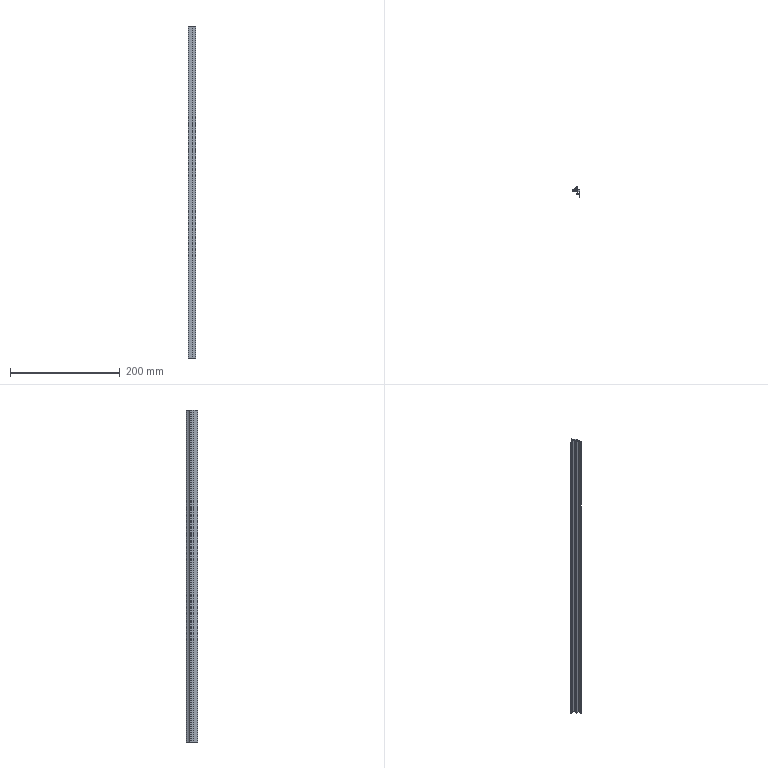Part | SolidWorks | features BaseBody 1, ICE 1, MoveFace 1 | 1 solid | 27 faces | box 14 x 20.3 x 606 mm | volume 30855 mm3 | plane 20 | cylinder 7 | commonest cylinder face diameters 0.387 x2 0.8 x2 0.4 x1 20 x1 22 x1
STEP:
#1=CARTESIAN_POINT('',(-5.304,-0.625,200.));
#2=VERTEX_POINT('',#1);
#3=CARTESIAN_POINT('',(-5.449,-0.8125,200.));
#4=VERTEX_POINT('',#3);
#5=CARTESIAN_POINT('',(-5.255,-0.8125,200.));
#6=DIRECTION('',(0.,0.,1.));
#7=DIRECTION('',(-1.,0.,0.));
#8=AXIS2_PLACEMENT_3D('',#5,#6,#7);
#9=CIRCLE('',#8,0.1937);
#10=EDGE_CURVE('',#2,#4,#9,.T.);
#11=ORIENTED_EDGE('',*,*,#10,.T.);
#12=CARTESIAN_POINT('',(-5.449,-0.8125,-406.));
#13=VERTEX_POINT('',#12);
#14=CARTESIAN_POINT('',(-5.449,-0.8125,230.));
#15=DIRECTION('',(0.,0.,-1.));
#16=VECTOR('',#15,1000.);
#17=LINE('',#14,#16);
#18=EDGE_CURVE('',#4,#13,#17,.T.);
#19=ORIENTED_EDGE('',*,*,#18,.T.);
#20=CARTESIAN_POINT('',(-5.304,-0.625,-406.));
#21=VERTEX_POINT('',#20);
#22=CARTESIAN_POINT('',(-5.255,-0.8125,-406.));
#23=DIRECTION('',(0.,0.,-1.));
#24=DIRECTION('',(1.,0.,0.));
#25=AXIS2_PLACEMENT_3D('',#22,#23,#24);
#26=CIRCLE('',#25,0.1937);
#27=EDGE_CURVE('',#13,#21,#26,.T.);
#28=ORIENTED_EDGE('',*,*,#27,.T.);
#29=CARTESIAN_POINT('',(-5.304,-0.625,230.));
#30=DIRECTION('',(0.,0.,-1.));
#31=VECTOR('',#30,1000.);
#32=LINE('',#29,#31);
#33=EDGE_CURVE('',#2,#21,#32,.T.);
#34=ORIENTED_EDGE('',*,*,#33,.F.);
#35=EDGE_LOOP('',(#11,#19,#28,#34));
#36=FACE_OUTER_BOUND('',#35,.T.);
#37=CARTESIAN_POINT('',(-5.255,-0.8125,230.));
#38=DIRECTION('',(0.,0.,-1.));
#39=DIRECTION('',(-1.,0.,0.));
#40=AXIS2_PLACEMENT_3D('',#37,#38,#39);
#41=CYLINDRICAL_SURFACE('',#40,0.1937);
#42=ADVANCED_FACE('',(#36),#41,.F.);
#43=CARTESIAN_POINT('',(5.,-1.,-406.));
#44=VERTEX_POINT('',#43);
#45=CARTESIAN_POINT('',(5.,-14.3,-406.));
#46=VERTEX_POINT('',#45);
#47=CARTESIAN_POINT('',(5.,29.623,-406.));
#48=DIRECTION('',(0.,-1.,0.));
#49=VECTOR('',#48,1000.);
#50=LINE('',#47,#49);
#51=EDGE_CURVE('',#44,#46,#50,.T.);
#52=ORIENTED_EDGE('',*,*,#51,.F.);
#53=CARTESIAN_POINT('',(5.,-1.,200.));
#54=VERTEX_POINT('',#53);
#55=CARTESIAN_POINT('',(5.,-1.,230.));
#56=DIRECTION('',(0.,0.,-1.));
#57=VECTOR('',#56,1000.);
#58=LINE('',#55,#57);
#59=EDGE_CURVE('',#54,#44,#58,.T.);
#60=ORIENTED_EDGE('',*,*,#59,.F.);
#61=CARTESIAN_POINT('',(5.,-14.3,200.));
#62=VERTEX_POINT('',#61);
#63=CARTESIAN_POINT('',(5.,-14.3,200.));
#64=DIRECTION('',(0.,1.,0.));
#65=VECTOR('',#64,1000.);
#66=LINE('',#63,#65);
#67=EDGE_CURVE('',#62,#54,#66,.T.);
#68=ORIENTED_EDGE('',*,*,#67,.F.);
#69=CARTESIAN_POINT('',(5.,-14.3,230.));
#70=DIRECTION('',(0.,0.,1.));
#71=VECTOR('',#70,1000.);
#72=LINE('',#69,#71);
#73=EDGE_CURVE('',#46,#62,#72,.T.);
#74=ORIENTED_EDGE('',*,*,#73,.F.);
#75=EDGE_LOOP('',(#52,#60,#68,#74));
#76=FACE_OUTER_BOUND('',#75,.T.);
#77=CARTESIAN_POINT('',(5.,-14.3,230.));
#78=DIRECTION('',(-1.,0.,0.));
#79=DIRECTION('',(0.,0.,1.));
#80=AXIS2_PLACEMENT_3D('',#77,#78,#79);
#81=PLANE('',#80);
#82=ADVANCED_FACE('',(#76),#81,.F.);
#83=CARTESIAN_POINT('',(-9.,-2.,-406.));
#84=VERTEX_POINT('',#83);
#85=CARTESIAN_POINT('',(-9.,-2.,200.));
#86=VERTEX_POINT('',#85);
#87=CARTESIAN_POINT('',(-9.,-2.,230.));
#88=DIRECTION('',(0.,0.,1.));
#89=VECTOR('',#88,1000.);
#90=LINE('',#87,#89);
#91=EDGE_CURVE('',#84,#86,#90,.T.);
#92=ORIENTED_EDGE('',*,*,#91,.F.);
#93=CARTESIAN_POINT('',(0.9,-2.,-406.));
#94=VERTEX_POINT('',#93);
#95=CARTESIAN_POINT('',(5.,-2.,-406.));
#96=DIRECTION('',(-1.,0.,0.));
#97=VECTOR('',#96,1000.);
#98=LINE('',#95,#97);
#99=EDGE_CURVE('',#94,#84,#98,.T.);
#100=ORIENTED_EDGE('',*,*,#99,.F.);
#101=CARTESIAN_POINT('',(0.9,-2.,200.));
#102=VERTEX_POINT('',#101);
#103=CARTESIAN_POINT('',(0.9,-2.,230.));
#104=DIRECTION('',(0.,0.,-1.));
#105=VECTOR('',#104,1000.);
#106=LINE('',#103,#105);
#107=EDGE_CURVE('',#102,#94,#106,.T.);
#108=ORIENTED_EDGE('',*,*,#107,.F.);
#109=CARTESIAN_POINT('',(5.,-2.,200.));
#110=DIRECTION('',(1.,0.,0.));
#111=VECTOR('',#110,1000.);
#112=LINE('',#109,#111);
#113=EDGE_CURVE('',#86,#102,#112,.T.);
#114=ORIENTED_EDGE('',*,*,#113,.F.);
#115=EDGE_LOOP('',(#92,#100,#108,#114));
#116=FACE_OUTER_BOUND('',#115,.T.);
#117=CARTESIAN_POINT('',(-9.,-2.,230.));
#118=DIRECTION('',(0.,1.,0.));
#119=DIRECTION('',(0.,0.,1.));
#120=AXIS2_PLACEMENT_3D('',#117,#118,#119);
#121=PLANE('',#120);
#122=ADVANCED_FACE('',(#116),#121,.F.);
#123=CARTESIAN_POINT('',(4.,-6.,200.));
#124=VERTEX_POINT('',#123);
#125=CARTESIAN_POINT('',(4.,-3.,200.));
#126=VERTEX_POINT('',#125);
#127=CARTESIAN_POINT('',(4.,29.623,200.));
#128=DIRECTION('',(0.,1.,0.));
#129=VECTOR('',#128,1000.);
#130=LINE('',#127,#129);
#131=EDGE_CURVE('',#124,#126,#130,.T.);
#132=ORIENTED_EDGE('',*,*,#131,.F.);
#133=CARTESIAN_POINT('',(1.,-6.,200.));
#134=VERTEX_POINT('',#133);
#135=CARTESIAN_POINT('',(5.,-6.,200.));
#136=DIRECTION('',(1.,0.,0.));
#137=VECTOR('',#136,1000.);
#138=LINE('',#135,#137);
#139=EDGE_CURVE('',#134,#124,#138,.T.);
#140=ORIENTED_EDGE('',*,*,#139,.F.);
#141=CARTESIAN_POINT('',(1.,-6.7,200.));
#142=VERTEX_POINT('',#141);
#143=CARTESIAN_POINT('',(1.,-6.,200.));
#144=DIRECTION('',(0.,-1.,0.));
#145=VECTOR('',#144,1000.);
#146=LINE('',#143,#145);
#147=EDGE_CURVE('',#134,#142,#146,.T.);
#148=ORIENTED_EDGE('',*,*,#147,.T.);
#149=CARTESIAN_POINT('',(-1.7,-6.7,200.));
#150=VERTEX_POINT('',#149);
#151=CARTESIAN_POINT('',(5.,-6.7,200.));
#152=DIRECTION('',(1.,0.,0.));
#153=VECTOR('',#152,1000.);
#154=LINE('',#151,#153);
#155=EDGE_CURVE('',#150,#142,#154,.T.);
#156=ORIENTED_EDGE('',*,*,#155,.F.);
#157=CARTESIAN_POINT('',(-1.7,-7.7,200.));
#158=VERTEX_POINT('',#157);
#159=CARTESIAN_POINT('',(-1.7,-6.7,200.));
#160=DIRECTION('',(0.,-1.,0.));
#161=VECTOR('',#160,1000.);
#162=LINE('',#159,#161);
#163=EDGE_CURVE('',#150,#158,#162,.T.);
#164=ORIENTED_EDGE('',*,*,#163,.T.);
#165=CARTESIAN_POINT('',(4.,-7.7,200.));
#166=VERTEX_POINT('',#165);
#167=CARTESIAN_POINT('',(5.,-7.7,200.));
#168=DIRECTION('',(-1.,0.,0.));
#169=VECTOR('',#168,1000.);
#170=LINE('',#167,#169);
#171=EDGE_CURVE('',#166,#158,#170,.T.);
#172=ORIENTED_EDGE('',*,*,#171,.F.);
#173=CARTESIAN_POINT('',(4.,-14.3,200.));
#174=VERTEX_POINT('',#173);
#175=CARTESIAN_POINT('',(4.,29.623,200.));
#176=DIRECTION('',(0.,1.,0.));
#177=VECTOR('',#176,1000.);
#178=LINE('',#175,#177);
#179=EDGE_CURVE('',#174,#166,#178,.T.);
#180=ORIENTED_EDGE('',*,*,#179,.F.);
#181=CARTESIAN_POINT('',(5.,-14.3,200.));
#182=DIRECTION('',(-1.,0.,0.));
#183=VECTOR('',#182,1000.);
#184=LINE('',#181,#183);
#185=EDGE_CURVE('',#62,#174,#184,.T.);
#186=ORIENTED_EDGE('',*,*,#185,.F.);
#187=ORIENTED_EDGE('',*,*,#67,.T.);
#188=CARTESIAN_POINT('',(-5.207,-1.,200.));
#189=VERTEX_POINT('',#188);
#190=CARTESIAN_POINT('',(5.,-1.,200.));
#191=DIRECTION('',(1.,0.,0.));
#192=VECTOR('',#191,1000.);
#193=LINE('',#190,#192);
#194=EDGE_CURVE('',#189,#54,#193,.T.);
#195=ORIENTED_EDGE('',*,*,#194,.F.);
#196=CARTESIAN_POINT('',(-5.255,-0.8125,200.));
#197=DIRECTION('',(0.,0.,1.));
#198=DIRECTION('',(-1.,0.,0.));
#199=AXIS2_PLACEMENT_3D('',#196,#197,#198);
#200=CIRCLE('',#199,0.1937);
#201=EDGE_CURVE('',#4,#189,#200,.T.);
#202=ORIENTED_EDGE('',*,*,#201,.F.);
#203=ORIENTED_EDGE('',*,*,#10,.F.);
#204=CARTESIAN_POINT('',(-1.368,3.063,200.));
#205=VERTEX_POINT('',#204);
#206=CARTESIAN_POINT('',(-10.628,9.,200.));
#207=DIRECTION('',(0.,0.,1.));
#208=DIRECTION('',(-1.,0.,0.));
#209=AXIS2_PLACEMENT_3D('',#206,#207,#208);
#210=CIRCLE('',#209,11.);
#211=EDGE_CURVE('',#2,#205,#210,.T.);
#212=ORIENTED_EDGE('',*,*,#211,.T.);
#213=CARTESIAN_POINT('',(-1.,2.955,200.));
#214=VERTEX_POINT('',#213);
#215=CARTESIAN_POINT('',(-1.2,2.955,200.));
#216=DIRECTION('',(0.,0.,1.));
#217=DIRECTION('',(-1.,0.,0.));
#218=AXIS2_PLACEMENT_3D('',#215,#216,#217);
#219=CIRCLE('',#218,0.2);
#220=EDGE_CURVE('',#214,#205,#219,.T.);
#221=ORIENTED_EDGE('',*,*,#220,.F.);
#222=CARTESIAN_POINT('',(-1.,1.5,200.));
#223=VERTEX_POINT('',#222);
#224=CARTESIAN_POINT('',(-1.,2.955,200.));
#225=DIRECTION('',(0.,1.,0.));
#226=VECTOR('',#225,1000.);
#227=LINE('',#224,#226);
#228=EDGE_CURVE('',#223,#214,#227,.T.);
#229=ORIENTED_EDGE('',*,*,#228,.F.);
#230=CARTESIAN_POINT('',(0.,1.5,200.));
#231=VERTEX_POINT('',#230);
#232=CARTESIAN_POINT('',(-1.,1.5,200.));
#233=DIRECTION('',(-1.,0.,0.));
#234=VECTOR('',#233,1000.);
#235=LINE('',#232,#234);
#236=EDGE_CURVE('',#231,#223,#235,.T.);
#237=ORIENTED_EDGE('',*,*,#236,.F.);
#238=CARTESIAN_POINT('',(0.,6.,200.));
#239=VERTEX_POINT('',#238);
#240=CARTESIAN_POINT('',(0.,1.5,200.));
#241=DIRECTION('',(0.,-1.,0.));
#242=VECTOR('',#241,1000.);
#243=LINE('',#240,#242);
#244=EDGE_CURVE('',#239,#231,#243,.T.);
#245=ORIENTED_EDGE('',*,*,#244,.F.);
#246=CARTESIAN_POINT('',(-0.8,6.,200.));
#247=VERTEX_POINT('',#246);
#248=CARTESIAN_POINT('',(0.,6.,200.));
#249=DIRECTION('',(1.,0.,0.));
#250=VECTOR('',#249,1000.);
#251=LINE('',#248,#250);
#252=EDGE_CURVE('',#247,#239,#251,.T.);
#253=ORIENTED_EDGE('',*,*,#252,.F.);
#254=CARTESIAN_POINT('',(-1.178,5.731,200.));
#255=VERTEX_POINT('',#254);
#256=CARTESIAN_POINT('',(-0.8,5.6,200.));
#257=DIRECTION('',(0.,0.,1.));
#258=DIRECTION('',(-1.,0.,0.));
#259=AXIS2_PLACEMENT_3D('',#256,#257,#258);
#260=CIRCLE('',#259,0.4);
#261=EDGE_CURVE('',#247,#255,#260,.T.);
#262=ORIENTED_EDGE('',*,*,#261,.T.);
#263=CARTESIAN_POINT('',(-8.678,-0.8077,200.));
#264=VERTEX_POINT('',#263);
#265=CARTESIAN_POINT('',(-10.628,9.,200.));
#266=DIRECTION('',(0.,0.,1.));
#267=DIRECTION('',(-1.,0.,0.));
#268=AXIS2_PLACEMENT_3D('',#265,#266,#267);
#269=CIRCLE('',#268,10.);
#270=EDGE_CURVE('',#264,#255,#269,.T.);
#271=ORIENTED_EDGE('',*,*,#270,.F.);
#272=CARTESIAN_POINT('',(-9.,-1.2,200.));
#273=VERTEX_POINT('',#272);
#274=CARTESIAN_POINT('',(-8.6,-1.2,200.));
#275=DIRECTION('',(0.,0.,1.));
#276=DIRECTION('',(-1.,0.,0.));
#277=AXIS2_PLACEMENT_3D('',#274,#275,#276);
#278=CIRCLE('',#277,0.4);
#279=EDGE_CURVE('',#264,#273,#278,.T.);
#280=ORIENTED_EDGE('',*,*,#279,.T.);
#281=CARTESIAN_POINT('',(-9.,8.,200.));
#282=DIRECTION('',(0.,-1.,0.));
#283=VECTOR('',#282,1000.);
#284=LINE('',#281,#283);
#285=EDGE_CURVE('',#273,#86,#284,.T.);
#286=ORIENTED_EDGE('',*,*,#285,.T.);
#287=ORIENTED_EDGE('',*,*,#113,.T.);
#288=CARTESIAN_POINT('',(0.9,-3.,200.));
#289=VERTEX_POINT('',#288);
#290=CARTESIAN_POINT('',(0.9,29.623,200.));
#291=DIRECTION('',(0.,1.,0.));
#292=VECTOR('',#291,1000.);
#293=LINE('',#290,#292);
#294=EDGE_CURVE('',#289,#102,#293,.T.);
#295=ORIENTED_EDGE('',*,*,#294,.F.);
#296=CARTESIAN_POINT('',(5.,-3.,200.));
#297=DIRECTION('',(-1.,0.,0.));
#298=VECTOR('',#297,1000.);
#299=LINE('',#296,#298);
#300=EDGE_CURVE('',#126,#289,#299,.T.);
#301=ORIENTED_EDGE('',*,*,#300,.F.);
#302=EDGE_LOOP('',(#132,#140,#148,#156,#164,#172,#180,#186,#187,#195,#202,#203,#212,#221,#229,#237,#245,#253,#262,#271,#280,#286,#287,#295,#301));
#303=FACE_OUTER_BOUND('',#302,.T.);
#304=CARTESIAN_POINT('',(5.,29.623,200.));
#305=DIRECTION('',(0.,0.,-1.));
#306=DIRECTION('',(-1.,0.,0.));
#307=AXIS2_PLACEMENT_3D('',#304,#305,#306);
#308=PLANE('',#307);
#309=ADVANCED_FACE('',(#303),#308,.F.);
#310=ORIENTED_EDGE('',*,*,#185,.T.);
#311=CARTESIAN_POINT('',(4.,-14.3,-406.));
#312=VERTEX_POINT('',#311);
#313=CARTESIAN_POINT('',(4.,-14.3,230.));
#314=DIRECTION('',(0.,0.,1.));
#315=VECTOR('',#314,1000.);
#316=LINE('',#313,#315);
#317=EDGE_CURVE('',#312,#174,#316,.T.);
#318=ORIENTED_EDGE('',*,*,#317,.F.);
#319=CARTESIAN_POINT('',(5.,-14.3,-406.));
#320=DIRECTION('',(-1.,0.,0.));
#321=VECTOR('',#320,1000.);
#322=LINE('',#319,#321);
#323=EDGE_CURVE('',#46,#312,#322,.T.);
#324=ORIENTED_EDGE('',*,*,#323,.F.);
#325=ORIENTED_EDGE('',*,*,#73,.T.);
#326=EDGE_LOOP('',(#310,#318,#324,#325));
#327=FACE_OUTER_BOUND('',#326,.T.);
#328=CARTESIAN_POINT('',(4.,-14.3,230.));
#329=DIRECTION('',(0.,1.,0.));
#330=DIRECTION('',(0.,0.,1.));
#331=AXIS2_PLACEMENT_3D('',#328,#329,#330);
#332=PLANE('',#331);
#333=ADVANCED_FACE('',(#327),#332,.F.);
#334=ORIENTED_EDGE('',*,*,#51,.T.);
#335=ORIENTED_EDGE('',*,*,#323,.T.);
#336=CARTESIAN_POINT('',(4.,-7.7,-406.));
#337=VERTEX_POINT('',#336);
#338=CARTESIAN_POINT('',(4.,-7.7,-406.));
#339=DIRECTION('',(0.,-1.,0.));
#340=VECTOR('',#339,1000.);
#341=LINE('',#338,#340);
#342=EDGE_CURVE('',#337,#312,#341,.T.);
#343=ORIENTED_EDGE('',*,*,#342,.F.);
#344=CARTESIAN_POINT('',(-1.7,-7.7,-406.));
#345=VERTEX_POINT('',#344);
#346=CARTESIAN_POINT('',(-1.7,-7.7,-406.));
#347=DIRECTION('',(1.,0.,0.));
#348=VECTOR('',#347,1000.);
#349=LINE('',#346,#348);
#350=EDGE_CURVE('',#345,#337,#349,.T.);
#351=ORIENTED_EDGE('',*,*,#350,.F.);
#352=CARTESIAN_POINT('',(-1.7,-6.7,-406.));
#353=VERTEX_POINT('',#352);
#354=CARTESIAN_POINT('',(-1.7,29.623,-406.));
#355=DIRECTION('',(0.,1.,0.));
#356=VECTOR('',#355,1000.);
#357=LINE('',#354,#356);
#358=EDGE_CURVE('',#345,#353,#357,.T.);
#359=ORIENTED_EDGE('',*,*,#358,.T.);
#360=CARTESIAN_POINT('',(1.,-6.7,-406.));
#361=VERTEX_POINT('',#360);
#362=CARTESIAN_POINT('',(1.,-6.7,-406.));
#363=DIRECTION('',(-1.,0.,0.));
#364=VECTOR('',#363,1000.);
#365=LINE('',#362,#364);
#366=EDGE_CURVE('',#361,#353,#365,.T.);
#367=ORIENTED_EDGE('',*,*,#366,.F.);
#368=CARTESIAN_POINT('',(1.,-6.,-406.));
#369=VERTEX_POINT('',#368);
#370=CARTESIAN_POINT('',(1.,29.623,-406.));
#371=DIRECTION('',(0.,1.,0.));
#372=VECTOR('',#371,1000.);
#373=LINE('',#370,#372);
#374=EDGE_CURVE('',#361,#369,#373,.T.);
#375=ORIENTED_EDGE('',*,*,#374,.T.);
#376=CARTESIAN_POINT('',(4.,-6.,-406.));
#377=VERTEX_POINT('',#376);
#378=CARTESIAN_POINT('',(4.,-6.,-406.));
#379=DIRECTION('',(-1.,0.,0.));
#380=VECTOR('',#379,1000.);
#381=LINE('',#378,#380);
#382=EDGE_CURVE('',#377,#369,#381,.T.);
#383=ORIENTED_EDGE('',*,*,#382,.F.);
#384=CARTESIAN_POINT('',(4.,-3.,-406.));
#385=VERTEX_POINT('',#384);
#386=CARTESIAN_POINT('',(4.,-3.,-406.));
#387=DIRECTION('',(0.,-1.,0.));
#388=VECTOR('',#387,1000.);
#389=LINE('',#386,#388);
#390=EDGE_CURVE('',#385,#377,#389,.T.);
#391=ORIENTED_EDGE('',*,*,#390,.F.);
#392=CARTESIAN_POINT('',(0.9,-3.,-406.));
#393=VERTEX_POINT('',#392);
#394=CARTESIAN_POINT('',(0.9,-3.,-406.));
#395=DIRECTION('',(1.,0.,0.));
#396=VECTOR('',#395,1000.);
#397=LINE('',#394,#396);
#398=EDGE_CURVE('',#393,#385,#397,.T.);
#399=ORIENTED_EDGE('',*,*,#398,.F.);
#400=CARTESIAN_POINT('',(0.9,-2.,-406.));
#401=DIRECTION('',(0.,-1.,0.));
#402=VECTOR('',#401,1000.);
#403=LINE('',#400,#402);
#404=EDGE_CURVE('',#94,#393,#403,.T.);
#405=ORIENTED_EDGE('',*,*,#404,.F.);
#406=ORIENTED_EDGE('',*,*,#99,.T.);
#407=CARTESIAN_POINT('',(-9.,-1.2,-406.));
#408=VERTEX_POINT('',#407);
#409=CARTESIAN_POINT('',(-9.,-1.2,-406.));
#410=DIRECTION('',(0.,-1.,0.));
#411=VECTOR('',#410,1000.);
#412=LINE('',#409,#411);
#413=EDGE_CURVE('',#408,#84,#412,.T.);
#414=ORIENTED_EDGE('',*,*,#413,.F.);
#415=CARTESIAN_POINT('',(-8.678,-0.8077,-406.));
#416=VERTEX_POINT('',#415);
#417=CARTESIAN_POINT('',(-8.6,-1.2,-406.));
#418=DIRECTION('',(0.,0.,-1.));
#419=DIRECTION('',(1.,0.,0.));
#420=AXIS2_PLACEMENT_3D('',#417,#418,#419);
#421=CIRCLE('',#420,0.4);
#422=EDGE_CURVE('',#408,#416,#421,.T.);
#423=ORIENTED_EDGE('',*,*,#422,.T.);
#424=CARTESIAN_POINT('',(-1.178,5.731,-406.));
#425=VERTEX_POINT('',#424);
#426=CARTESIAN_POINT('',(-10.628,9.,-406.));
#427=DIRECTION('',(0.,0.,-1.));
#428=DIRECTION('',(1.,0.,0.));
#429=AXIS2_PLACEMENT_3D('',#426,#427,#428);
#430=CIRCLE('',#429,10.);
#431=EDGE_CURVE('',#425,#416,#430,.T.);
#432=ORIENTED_EDGE('',*,*,#431,.F.);
#433=CARTESIAN_POINT('',(-0.8,6.,-406.));
#434=VERTEX_POINT('',#433);
#435=CARTESIAN_POINT('',(-0.8,5.6,-406.));
#436=DIRECTION('',(0.,0.,-1.));
#437=DIRECTION('',(1.,0.,0.));
#438=AXIS2_PLACEMENT_3D('',#435,#436,#437);
#439=CIRCLE('',#438,0.4);
#440=EDGE_CURVE('',#425,#434,#439,.T.);
#441=ORIENTED_EDGE('',*,*,#440,.T.);
#442=CARTESIAN_POINT('',(0.,6.,-406.));
#443=VERTEX_POINT('',#442);
#444=CARTESIAN_POINT('',(0.,6.,-406.));
#445=DIRECTION('',(-1.,0.,0.));
#446=VECTOR('',#445,1000.);
#447=LINE('',#444,#446);
#448=EDGE_CURVE('',#443,#434,#447,.T.);
#449=ORIENTED_EDGE('',*,*,#448,.F.);
#450=CARTESIAN_POINT('',(0.,1.5,-406.));
#451=VERTEX_POINT('',#450);
#452=CARTESIAN_POINT('',(0.,1.5,-406.));
#453=DIRECTION('',(0.,1.,0.));
#454=VECTOR('',#453,1000.);
#455=LINE('',#452,#454);
#456=EDGE_CURVE('',#451,#443,#455,.T.);
#457=ORIENTED_EDGE('',*,*,#456,.F.);
#458=CARTESIAN_POINT('',(-1.,1.5,-406.));
#459=VERTEX_POINT('',#458);
#460=CARTESIAN_POINT('',(-1.,1.5,-406.));
#461=DIRECTION('',(1.,0.,0.));
#462=VECTOR('',#461,1000.);
#463=LINE('',#460,#462);
#464=EDGE_CURVE('',#459,#451,#463,.T.);
#465=ORIENTED_EDGE('',*,*,#464,.F.);
#466=CARTESIAN_POINT('',(-1.,2.955,-406.));
#467=VERTEX_POINT('',#466);
#468=CARTESIAN_POINT('',(-1.,2.955,-406.));
#469=DIRECTION('',(0.,-1.,0.));
#470=VECTOR('',#469,1000.);
#471=LINE('',#468,#470);
#472=EDGE_CURVE('',#467,#459,#471,.T.);
#473=ORIENTED_EDGE('',*,*,#472,.F.);
#474=CARTESIAN_POINT('',(-1.368,3.063,-406.));
#475=VERTEX_POINT('',#474);
#476=CARTESIAN_POINT('',(-1.2,2.955,-406.));
#477=DIRECTION('',(0.,0.,-1.));
#478=DIRECTION('',(1.,0.,0.));
#479=AXIS2_PLACEMENT_3D('',#476,#477,#478);
#480=CIRCLE('',#479,0.2);
#481=EDGE_CURVE('',#475,#467,#480,.T.);
#482=ORIENTED_EDGE('',*,*,#481,.F.);
#483=CARTESIAN_POINT('',(-10.628,9.,-406.));
#484=DIRECTION('',(0.,0.,-1.));
#485=DIRECTION('',(1.,0.,0.));
#486=AXIS2_PLACEMENT_3D('',#483,#484,#485);
#487=CIRCLE('',#486,11.);
#488=EDGE_CURVE('',#475,#21,#487,.T.);
#489=ORIENTED_EDGE('',*,*,#488,.T.);
#490=ORIENTED_EDGE('',*,*,#27,.F.);
#491=CARTESIAN_POINT('',(-5.207,-1.,-406.));
#492=VERTEX_POINT('',#491);
#493=CARTESIAN_POINT('',(-5.255,-0.8125,-406.));
#494=DIRECTION('',(0.,0.,-1.));
#495=DIRECTION('',(1.,0.,0.));
#496=AXIS2_PLACEMENT_3D('',#493,#494,#495);
#497=CIRCLE('',#496,0.1937);
#498=EDGE_CURVE('',#492,#13,#497,.T.);
#499=ORIENTED_EDGE('',*,*,#498,.F.);
#500=CARTESIAN_POINT('',(5.,-1.,-406.));
#501=DIRECTION('',(-1.,0.,0.));
#502=VECTOR('',#501,1000.);
#503=LINE('',#500,#502);
#504=EDGE_CURVE('',#44,#492,#503,.T.);
#505=ORIENTED_EDGE('',*,*,#504,.F.);
#506=EDGE_LOOP('',(#334,#335,#343,#351,#359,#367,#375,#383,#391,#399,#405,#406,#414,#423,#432,#441,#449,#457,#465,#473,#482,#489,#490,#499,#505));
#507=FACE_OUTER_BOUND('',#506,.T.);
#508=CARTESIAN_POINT('',(5.,29.623,-406.));
#509=DIRECTION('',(0.,0.,1.));
#510=DIRECTION('',(1.,0.,0.));
#511=AXIS2_PLACEMENT_3D('',#508,#509,#510);
#512=PLANE('',#511);
#513=ADVANCED_FACE('',(#507),#512,.F.);
#514=ORIENTED_EDGE('',*,*,#59,.T.);
#515=ORIENTED_EDGE('',*,*,#504,.T.);
#516=CARTESIAN_POINT('',(-5.207,-1.,230.));
#517=DIRECTION('',(0.,0.,-1.));
#518=VECTOR('',#517,1000.);
#519=LINE('',#516,#518);
#520=EDGE_CURVE('',#189,#492,#519,.T.);
#521=ORIENTED_EDGE('',*,*,#520,.F.);
#522=ORIENTED_EDGE('',*,*,#194,.T.);
#523=EDGE_LOOP('',(#514,#515,#521,#522));
#524=FACE_OUTER_BOUND('',#523,.T.);
#525=CARTESIAN_POINT('',(5.,-1.,230.));
#526=DIRECTION('',(0.,-1.,0.));
#527=DIRECTION('',(0.,0.,-1.));
#528=AXIS2_PLACEMENT_3D('',#525,#526,#527);
#529=PLANE('',#528);
#530=ADVANCED_FACE('',(#524),#529,.F.);
#531=CARTESIAN_POINT('',(-9.,-1.2,230.));
#532=DIRECTION('',(0.,0.,1.));
#533=VECTOR('',#532,1000.);
#534=LINE('',#531,#533);
#535=EDGE_CURVE('',#408,#273,#534,.T.);
#536=ORIENTED_EDGE('',*,*,#535,.F.);
#537=ORIENTED_EDGE('',*,*,#413,.T.);
#538=ORIENTED_EDGE('',*,*,#91,.T.);
#539=ORIENTED_EDGE('',*,*,#285,.F.);
#540=EDGE_LOOP('',(#536,#537,#538,#539));
#541=FACE_OUTER_BOUND('',#540,.T.);
#542=CARTESIAN_POINT('',(-9.,-1.2,230.));
#543=DIRECTION('',(1.,0.,0.));
#544=DIRECTION('',(0.,0.,-1.));
#545=AXIS2_PLACEMENT_3D('',#542,#543,#544);
#546=PLANE('',#545);
#547=ADVANCED_FACE('',(#541),#546,.F.);
#548=ORIENTED_EDGE('',*,*,#294,.T.);
#549=ORIENTED_EDGE('',*,*,#107,.T.);
#550=ORIENTED_EDGE('',*,*,#404,.T.);
#551=CARTESIAN_POINT('',(0.9,-3.,230.));
#552=DIRECTION('',(0.,0.,-1.));
#553=VECTOR('',#552,1000.);
#554=LINE('',#551,#553);
#555=EDGE_CURVE('',#289,#393,#554,.T.);
#556=ORIENTED_EDGE('',*,*,#555,.F.);
#557=EDGE_LOOP('',(#548,#549,#550,#556));
#558=FACE_OUTER_BOUND('',#557,.T.);
#559=CARTESIAN_POINT('',(0.9,-2.,230.));
#560=DIRECTION('',(1.,0.,0.));
#561=DIRECTION('',(0.,0.,-1.));
#562=AXIS2_PLACEMENT_3D('',#559,#560,#561);
#563=PLANE('',#562);
#564=ADVANCED_FACE('',(#558),#563,.F.);
#565=ORIENTED_EDGE('',*,*,#300,.T.);
#566=ORIENTED_EDGE('',*,*,#555,.T.);
#567=ORIENTED_EDGE('',*,*,#398,.T.);
#568=CARTESIAN_POINT('',(4.,-3.,230.));
#569=DIRECTION('',(0.,0.,-1.));
#570=VECTOR('',#569,1000.);
#571=LINE('',#568,#570);
#572=EDGE_CURVE('',#126,#385,#571,.T.);
#573=ORIENTED_EDGE('',*,*,#572,.F.);
#574=EDGE_LOOP('',(#565,#566,#567,#573));
#575=FACE_OUTER_BOUND('',#574,.T.);
#576=CARTESIAN_POINT('',(0.9,-3.,230.));
#577=DIRECTION('',(0.,1.,0.));
#578=DIRECTION('',(0.,0.,1.));
#579=AXIS2_PLACEMENT_3D('',#576,#577,#578);
#580=PLANE('',#579);
#581=ADVANCED_FACE('',(#575),#580,.F.);
#582=ORIENTED_EDGE('',*,*,#131,.T.);
#583=ORIENTED_EDGE('',*,*,#572,.T.);
#584=ORIENTED_EDGE('',*,*,#390,.T.);
#585=CARTESIAN_POINT('',(4.,-6.,230.));
#586=DIRECTION('',(0.,0.,-1.));
#587=VECTOR('',#586,1000.);
#588=LINE('',#585,#587);
#589=EDGE_CURVE('',#124,#377,#588,.T.);
#590=ORIENTED_EDGE('',*,*,#589,.F.);
#591=EDGE_LOOP('',(#582,#583,#584,#590));
#592=FACE_OUTER_BOUND('',#591,.T.);
#593=CARTESIAN_POINT('',(4.,-3.,230.));
#594=DIRECTION('',(1.,0.,0.));
#595=DIRECTION('',(0.,0.,-1.));
#596=AXIS2_PLACEMENT_3D('',#593,#594,#595);
#597=PLANE('',#596);
#598=ADVANCED_FACE('',(#592),#597,.F.);
#599=ORIENTED_EDGE('',*,*,#139,.T.);
#600=ORIENTED_EDGE('',*,*,#589,.T.);
#601=ORIENTED_EDGE('',*,*,#382,.T.);
#602=CARTESIAN_POINT('',(1.,-6.,230.));
#603=DIRECTION('',(0.,0.,-1.));
#604=VECTOR('',#603,1000.);
#605=LINE('',#602,#604);
#606=EDGE_CURVE('',#134,#369,#605,.T.);
#607=ORIENTED_EDGE('',*,*,#606,.F.);
#608=EDGE_LOOP('',(#599,#600,#601,#607));
#609=FACE_OUTER_BOUND('',#608,.T.);
#610=CARTESIAN_POINT('',(4.,-6.,230.));
#611=DIRECTION('',(0.,-1.,0.));
#612=DIRECTION('',(0.,0.,-1.));
#613=AXIS2_PLACEMENT_3D('',#610,#611,#612);
#614=PLANE('',#613);
#615=ADVANCED_FACE('',(#609),#614,.F.);
#616=ORIENTED_EDGE('',*,*,#155,.T.);
#617=CARTESIAN_POINT('',(1.,-6.7,230.));
#618=DIRECTION('',(0.,0.,1.));
#619=VECTOR('',#618,1000.);
#620=LINE('',#617,#619);
#621=EDGE_CURVE('',#361,#142,#620,.T.);
#622=ORIENTED_EDGE('',*,*,#621,.F.);
#623=ORIENTED_EDGE('',*,*,#366,.T.);
#624=CARTESIAN_POINT('',(-1.7,-6.7,230.));
#625=DIRECTION('',(0.,0.,-1.));
#626=VECTOR('',#625,1000.);
#627=LINE('',#624,#626);
#628=EDGE_CURVE('',#150,#353,#627,.T.);
#629=ORIENTED_EDGE('',*,*,#628,.F.);
#630=EDGE_LOOP('',(#616,#622,#623,#629));
#631=FACE_OUTER_BOUND('',#630,.T.);
#632=CARTESIAN_POINT('',(1.,-6.7,230.));
#633=DIRECTION('',(0.,-1.,0.));
#634=DIRECTION('',(0.,0.,-1.));
#635=AXIS2_PLACEMENT_3D('',#632,#633,#634);
#636=PLANE('',#635);
#637=ADVANCED_FACE('',(#631),#636,.F.);
#638=ORIENTED_EDGE('',*,*,#171,.T.);
#639=CARTESIAN_POINT('',(-1.7,-7.7,230.));
#640=DIRECTION('',(0.,0.,1.));
#641=VECTOR('',#640,1000.);
#642=LINE('',#639,#641);
#643=EDGE_CURVE('',#345,#158,#642,.T.);
#644=ORIENTED_EDGE('',*,*,#643,.F.);
#645=ORIENTED_EDGE('',*,*,#350,.T.);
#646=CARTESIAN_POINT('',(4.,-7.7,230.));
#647=DIRECTION('',(0.,0.,-1.));
#648=VECTOR('',#647,1000.);
#649=LINE('',#646,#648);
#650=EDGE_CURVE('',#166,#337,#649,.T.);
#651=ORIENTED_EDGE('',*,*,#650,.F.);
#652=EDGE_LOOP('',(#638,#644,#645,#651));
#653=FACE_OUTER_BOUND('',#652,.T.);
#654=CARTESIAN_POINT('',(-1.7,-7.7,230.));
#655=DIRECTION('',(0.,1.,0.));
#656=DIRECTION('',(0.,0.,1.));
#657=AXIS2_PLACEMENT_3D('',#654,#655,#656);
#658=PLANE('',#657);
#659=ADVANCED_FACE('',(#653),#658,.F.);
#660=ORIENTED_EDGE('',*,*,#179,.T.);
#661=ORIENTED_EDGE('',*,*,#650,.T.);
#662=ORIENTED_EDGE('',*,*,#342,.T.);
#663=ORIENTED_EDGE('',*,*,#317,.T.);
#664=EDGE_LOOP('',(#660,#661,#662,#663));
#665=FACE_OUTER_BOUND('',#664,.T.);
#666=CARTESIAN_POINT('',(4.,-7.7,230.));
#667=DIRECTION('',(1.,0.,0.));
#668=DIRECTION('',(0.,0.,-1.));
#669=AXIS2_PLACEMENT_3D('',#666,#667,#668);
#670=PLANE('',#669);
#671=ADVANCED_FACE('',(#665),#670,.F.);
#672=ORIENTED_EDGE('',*,*,#18,.F.);
#673=ORIENTED_EDGE('',*,*,#201,.T.);
#674=ORIENTED_EDGE('',*,*,#520,.T.);
#675=ORIENTED_EDGE('',*,*,#498,.T.);
#676=EDGE_LOOP('',(#672,#673,#674,#675));
#677=FACE_OUTER_BOUND('',#676,.T.);
#678=CARTESIAN_POINT('',(-5.255,-0.8125,230.));
#679=DIRECTION('',(0.,0.,-1.));
#680=DIRECTION('',(-1.,0.,0.));
#681=AXIS2_PLACEMENT_3D('',#678,#679,#680);
#682=CYLINDRICAL_SURFACE('',#681,0.1937);
#683=ADVANCED_FACE('',(#677),#682,.F.);
#684=CARTESIAN_POINT('',(-1.,2.955,230.));
#685=DIRECTION('',(0.,0.,1.));
#686=VECTOR('',#685,1000.);
#687=LINE('',#684,#686);
#688=EDGE_CURVE('',#467,#214,#687,.T.);
#689=ORIENTED_EDGE('',*,*,#688,.F.);
#690=ORIENTED_EDGE('',*,*,#472,.T.);
#691=CARTESIAN_POINT('',(-1.,1.5,230.));
#692=DIRECTION('',(0.,0.,-1.));
#693=VECTOR('',#692,1000.);
#694=LINE('',#691,#693);
#695=EDGE_CURVE('',#223,#459,#694,.T.);
#696=ORIENTED_EDGE('',*,*,#695,.F.);
#697=ORIENTED_EDGE('',*,*,#228,.T.);
#698=EDGE_LOOP('',(#689,#690,#696,#697));
#699=FACE_OUTER_BOUND('',#698,.T.);
#700=CARTESIAN_POINT('',(-1.,2.955,230.));
#701=DIRECTION('',(1.,0.,0.));
#702=DIRECTION('',(0.,0.,-1.));
#703=AXIS2_PLACEMENT_3D('',#700,#701,#702);
#704=PLANE('',#703);
#705=ADVANCED_FACE('',(#699),#704,.F.);
#706=ORIENTED_EDGE('',*,*,#488,.F.);
#707=CARTESIAN_POINT('',(-1.368,3.063,230.));
#708=DIRECTION('',(0.,0.,1.));
#709=VECTOR('',#708,1000.);
#710=LINE('',#707,#709);
#711=EDGE_CURVE('',#475,#205,#710,.T.);
#712=ORIENTED_EDGE('',*,*,#711,.T.);
#713=ORIENTED_EDGE('',*,*,#211,.F.);
#714=ORIENTED_EDGE('',*,*,#33,.T.);
#715=EDGE_LOOP('',(#706,#712,#713,#714));
#716=FACE_OUTER_BOUND('',#715,.T.);
#717=CARTESIAN_POINT('',(-10.628,9.,230.));
#718=DIRECTION('',(0.,0.,-1.));
#719=DIRECTION('',(-1.,0.,0.));
#720=AXIS2_PLACEMENT_3D('',#717,#718,#719);
#721=CYLINDRICAL_SURFACE('',#720,11.);
#722=ADVANCED_FACE('',(#716),#721,.T.);
#723=CARTESIAN_POINT('',(-1.178,5.731,230.));
#724=DIRECTION('',(0.,0.,1.));
#725=VECTOR('',#724,1000.);
#726=LINE('',#723,#725);
#727=EDGE_CURVE('',#425,#255,#726,.T.);
#728=ORIENTED_EDGE('',*,*,#727,.F.);
#729=ORIENTED_EDGE('',*,*,#431,.T.);
#730=CARTESIAN_POINT('',(-8.678,-0.8077,230.));
#731=DIRECTION('',(0.,0.,-1.));
#732=VECTOR('',#731,1000.);
#733=LINE('',#730,#732);
#734=EDGE_CURVE('',#264,#416,#733,.T.);
#735=ORIENTED_EDGE('',*,*,#734,.F.);
#736=ORIENTED_EDGE('',*,*,#270,.T.);
#737=EDGE_LOOP('',(#728,#729,#735,#736));
#738=FACE_OUTER_BOUND('',#737,.T.);
#739=CARTESIAN_POINT('',(-10.628,9.,230.));
#740=DIRECTION('',(0.,0.,-1.));
#741=DIRECTION('',(-1.,0.,0.));
#742=AXIS2_PLACEMENT_3D('',#739,#740,#741);
#743=CYLINDRICAL_SURFACE('',#742,10.);
#744=ADVANCED_FACE('',(#738),#743,.F.);
#745=CARTESIAN_POINT('',(0.,1.5,230.));
#746=DIRECTION('',(0.,0.,1.));
#747=VECTOR('',#746,1000.);
#748=LINE('',#745,#747);
#749=EDGE_CURVE('',#451,#231,#748,.T.);
#750=ORIENTED_EDGE('',*,*,#749,.F.);
#751=ORIENTED_EDGE('',*,*,#456,.T.);
#752=CARTESIAN_POINT('',(0.,6.,230.));
#753=DIRECTION('',(0.,0.,-1.));
#754=VECTOR('',#753,1000.);
#755=LINE('',#752,#754);
#756=EDGE_CURVE('',#239,#443,#755,.T.);
#757=ORIENTED_EDGE('',*,*,#756,.F.);
#758=ORIENTED_EDGE('',*,*,#244,.T.);
#759=EDGE_LOOP('',(#750,#751,#757,#758));
#760=FACE_OUTER_BOUND('',#759,.T.);
#761=CARTESIAN_POINT('',(0.,1.5,230.));
#762=DIRECTION('',(-1.,0.,0.));
#763=DIRECTION('',(0.,0.,1.));
#764=AXIS2_PLACEMENT_3D('',#761,#762,#763);
#765=PLANE('',#764);
#766=ADVANCED_FACE('',(#760),#765,.F.);
#767=ORIENTED_EDGE('',*,*,#422,.F.);
#768=ORIENTED_EDGE('',*,*,#535,.T.);
#769=ORIENTED_EDGE('',*,*,#279,.F.);
#770=ORIENTED_EDGE('',*,*,#734,.T.);
#771=EDGE_LOOP('',(#767,#768,#769,#770));
#772=FACE_OUTER_BOUND('',#771,.T.);
#773=CARTESIAN_POINT('',(-8.6,-1.2,230.));
#774=DIRECTION('',(0.,0.,-1.));
#775=DIRECTION('',(-1.,0.,0.));
#776=AXIS2_PLACEMENT_3D('',#773,#774,#775);
#777=CYLINDRICAL_SURFACE('',#776,0.4);
#778=ADVANCED_FACE('',(#772),#777,.T.);
#779=ORIENTED_EDGE('',*,*,#147,.F.);
#780=ORIENTED_EDGE('',*,*,#606,.T.);
#781=ORIENTED_EDGE('',*,*,#374,.F.);
#782=ORIENTED_EDGE('',*,*,#621,.T.);
#783=EDGE_LOOP('',(#779,#780,#781,#782));
#784=FACE_OUTER_BOUND('',#783,.T.);
#785=CARTESIAN_POINT('',(1.,-6.,230.));
#786=DIRECTION('',(1.,0.,0.));
#787=DIRECTION('',(0.,0.,-1.));
#788=AXIS2_PLACEMENT_3D('',#785,#786,#787);
#789=PLANE('',#788);
#790=ADVANCED_FACE('',(#784),#789,.F.);
#791=ORIENTED_EDGE('',*,*,#163,.F.);
#792=ORIENTED_EDGE('',*,*,#628,.T.);
#793=ORIENTED_EDGE('',*,*,#358,.F.);
#794=ORIENTED_EDGE('',*,*,#643,.T.);
#795=EDGE_LOOP('',(#791,#792,#793,#794));
#796=FACE_OUTER_BOUND('',#795,.T.);
#797=CARTESIAN_POINT('',(-1.7,-6.7,230.));
#798=DIRECTION('',(1.,0.,0.));
#799=DIRECTION('',(0.,0.,-1.));
#800=AXIS2_PLACEMENT_3D('',#797,#798,#799);
#801=PLANE('',#800);
#802=ADVANCED_FACE('',(#796),#801,.F.);
#803=ORIENTED_EDGE('',*,*,#711,.F.);
#804=ORIENTED_EDGE('',*,*,#481,.T.);
#805=ORIENTED_EDGE('',*,*,#688,.T.);
#806=ORIENTED_EDGE('',*,*,#220,.T.);
#807=EDGE_LOOP('',(#803,#804,#805,#806));
#808=FACE_OUTER_BOUND('',#807,.T.);
#809=CARTESIAN_POINT('',(-1.2,2.955,230.));
#810=DIRECTION('',(0.,0.,-1.));
#811=DIRECTION('',(-1.,0.,0.));
#812=AXIS2_PLACEMENT_3D('',#809,#810,#811);
#813=CYLINDRICAL_SURFACE('',#812,0.2);
#814=ADVANCED_FACE('',(#808),#813,.F.);
#815=ORIENTED_EDGE('',*,*,#695,.T.);
#816=ORIENTED_EDGE('',*,*,#464,.T.);
#817=ORIENTED_EDGE('',*,*,#749,.T.);
#818=ORIENTED_EDGE('',*,*,#236,.T.);
#819=EDGE_LOOP('',(#815,#816,#817,#818));
#820=FACE_OUTER_BOUND('',#819,.T.);
#821=CARTESIAN_POINT('',(-1.,1.5,230.));
#822=DIRECTION('',(0.,1.,0.));
#823=DIRECTION('',(0.,0.,1.));
#824=AXIS2_PLACEMENT_3D('',#821,#822,#823);
#825=PLANE('',#824);
#826=ADVANCED_FACE('',(#820),#825,.F.);
#827=ORIENTED_EDGE('',*,*,#440,.F.);
#828=ORIENTED_EDGE('',*,*,#727,.T.);
#829=ORIENTED_EDGE('',*,*,#261,.F.);
#830=CARTESIAN_POINT('',(-0.8,6.,230.));
#831=DIRECTION('',(0.,0.,-1.));
#832=VECTOR('',#831,1000.);
#833=LINE('',#830,#832);
#834=EDGE_CURVE('',#247,#434,#833,.T.);
#835=ORIENTED_EDGE('',*,*,#834,.T.);
#836=EDGE_LOOP('',(#827,#828,#829,#835));
#837=FACE_OUTER_BOUND('',#836,.T.);
#838=CARTESIAN_POINT('',(-0.8,5.6,230.));
#839=DIRECTION('',(0.,0.,-1.));
#840=DIRECTION('',(-1.,0.,0.));
#841=AXIS2_PLACEMENT_3D('',#838,#839,#840);
#842=CYLINDRICAL_SURFACE('',#841,0.4);
#843=ADVANCED_FACE('',(#837),#842,.T.);
#844=ORIENTED_EDGE('',*,*,#756,.T.);
#845=ORIENTED_EDGE('',*,*,#448,.T.);
#846=ORIENTED_EDGE('',*,*,#834,.F.);
#847=ORIENTED_EDGE('',*,*,#252,.T.);
#848=EDGE_LOOP('',(#844,#845,#846,#847));
#849=FACE_OUTER_BOUND('',#848,.T.);
#850=CARTESIAN_POINT('',(0.,6.,230.));
#851=DIRECTION('',(0.,-1.,0.));
#852=DIRECTION('',(0.,0.,-1.));
#853=AXIS2_PLACEMENT_3D('',#850,#851,#852);
#854=PLANE('',#853);
#855=ADVANCED_FACE('',(#849),#854,.F.);
#856=CLOSED_SHELL('',(#42,#82,#122,#309,#333,#513,#530,#547,#564,#581,#598,#615,#637,#659,#671,#683,#705,#722,#744,#766,#778,#790,#802,#814,#826,#843,#855));
#857=MANIFOLD_SOLID_BREP('',#856);
#858=CARTESIAN_POINT('',(0.,0.,0.));
#859=DIRECTION('',(0.,0.,1.));
#860=DIRECTION('',(1.,0.,0.));
#861=AXIS2_PLACEMENT_3D('',#858,#859,#860);
#862=(LENGTH_UNIT()NAMED_UNIT(*)SI_UNIT(.MILLI.,.METRE.));
#863=UNCERTAINTY_MEASURE_WITH_UNIT(LENGTH_MEASURE(0.00001),#862,'','');
#864=(NAMED_UNIT(*)PLANE_ANGLE_UNIT()SI_UNIT($,.RADIAN.));
#865=(NAMED_UNIT(*)SI_UNIT($,.STERADIAN.)SOLID_ANGLE_UNIT());
#866=(GEOMETRIC_REPRESENTATION_CONTEXT(3)GLOBAL_UNCERTAINTY_ASSIGNED_CONTEXT((#863))GLOBAL_UNIT_ASSIGNED_CONTEXT((#862,#864,#865))REPRESENTATION_CONTEXT('',''));
#867=ADVANCED_BREP_SHAPE_REPRESENTATION('',(#857,#861),#866);